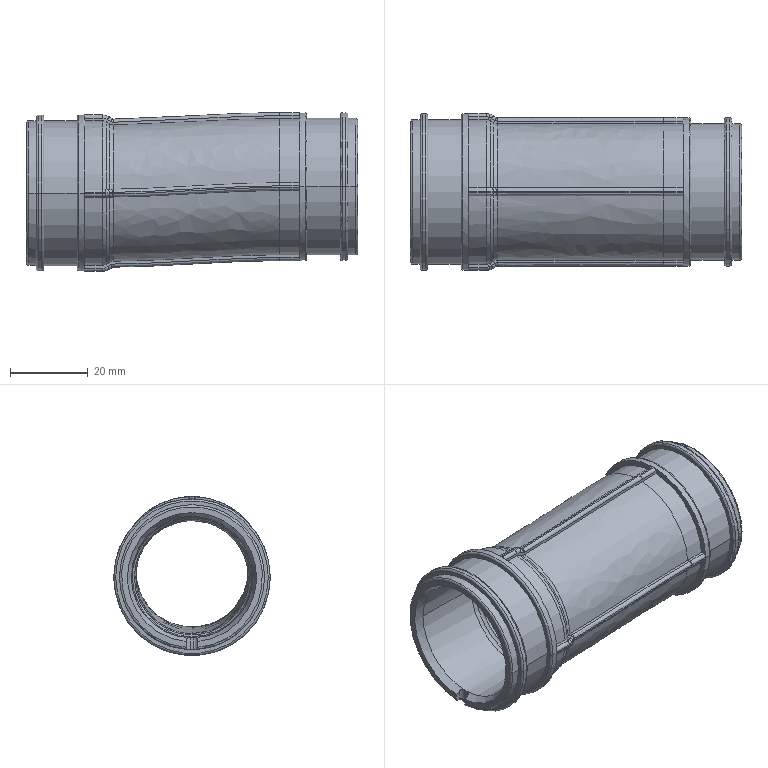Part | STEP file | ZXW722-L-92 | 1 solid | 201 faces | box 85 x 40.159 x 40.76 mm | volume 27832 mm3 | spline 77 | cylinder 53 | plane 41 | torus 21 | other 6 | cone 3 | commonest cylinder face diameters 1.6 x20 35 x8 37.159 x8 38 x4 40.159 x4 7 x3